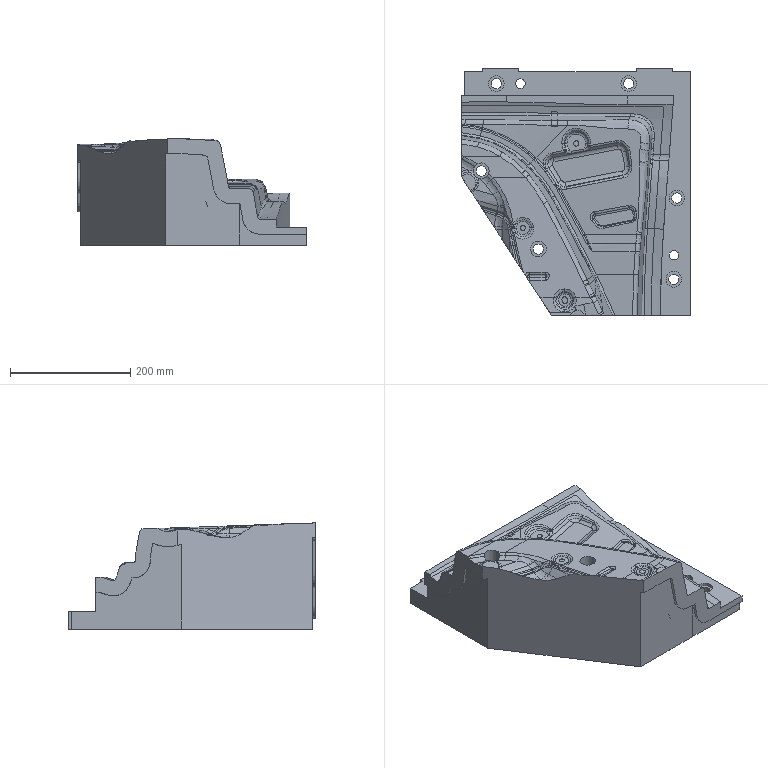Part | NX | features solid 2 | 1 solid | 351 faces | box 381.996 x 410 x 176.391 mm | volume 12374117 mm3 | spline 306 | plane 30 | cylinder 15 | commonest cylinder face diameters 26 x7 17 x6 16 x2